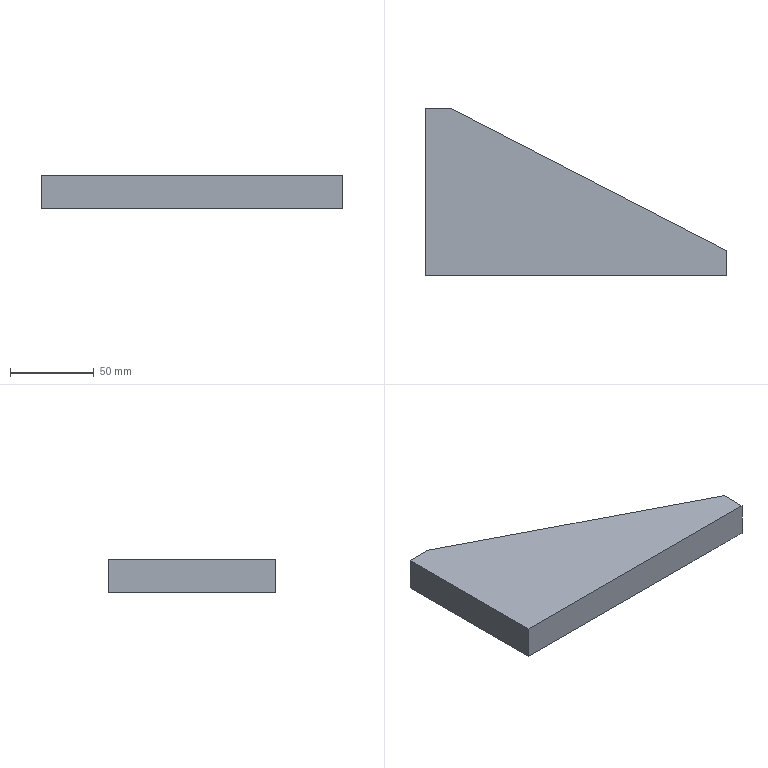Part | SolidWorks | features Extrusion 1 | 1 solid | 7 faces | box 180 x 100 x 20 mm | volume 219750 mm3 | plane 7
STEP:
#1=CARTESIAN_POINT('',(0.,0.,0.));
#2=VERTEX_POINT('',#1);
#3=CARTESIAN_POINT('',(180.,0.,0.));
#4=VERTEX_POINT('',#3);
#5=CARTESIAN_POINT('',(180.,0.,0.));
#6=DIRECTION('',(1.,0.,0.));
#7=VECTOR('',#6,1000.);
#8=LINE('',#5,#7);
#9=EDGE_CURVE('',#2,#4,#8,.T.);
#10=ORIENTED_EDGE('',*,*,#9,.T.);
#11=CARTESIAN_POINT('',(180.,0.,20.));
#12=VERTEX_POINT('',#11);
#13=CARTESIAN_POINT('',(180.,0.,20.));
#14=DIRECTION('',(0.,0.,-1.));
#15=VECTOR('',#14,1000.);
#16=LINE('',#13,#15);
#17=EDGE_CURVE('',#12,#4,#16,.T.);
#18=ORIENTED_EDGE('',*,*,#17,.F.);
#19=CARTESIAN_POINT('',(0.,0.,20.));
#20=VERTEX_POINT('',#19);
#21=CARTESIAN_POINT('',(180.,0.,20.));
#22=DIRECTION('',(1.,0.,0.));
#23=VECTOR('',#22,1000.);
#24=LINE('',#21,#23);
#25=EDGE_CURVE('',#20,#12,#24,.T.);
#26=ORIENTED_EDGE('',*,*,#25,.F.);
#27=CARTESIAN_POINT('',(0.,0.,20.));
#28=DIRECTION('',(0.,0.,-1.));
#29=VECTOR('',#28,1000.);
#30=LINE('',#27,#29);
#31=EDGE_CURVE('',#20,#2,#30,.T.);
#32=ORIENTED_EDGE('',*,*,#31,.T.);
#33=EDGE_LOOP('',(#10,#18,#26,#32));
#34=FACE_OUTER_BOUND('',#33,.T.);
#35=CARTESIAN_POINT('',(180.,0.,20.));
#36=DIRECTION('',(0.,1.,0.));
#37=DIRECTION('',(-1.,0.,0.));
#38=AXIS2_PLACEMENT_3D('',#35,#36,#37);
#39=PLANE('',#38);
#40=ADVANCED_FACE('',(#34),#39,.F.);
#41=CARTESIAN_POINT('',(180.,15.,0.));
#42=VERTEX_POINT('',#41);
#43=CARTESIAN_POINT('',(180.,15.,0.));
#44=DIRECTION('',(0.,1.,0.));
#45=VECTOR('',#44,1000.);
#46=LINE('',#43,#45);
#47=EDGE_CURVE('',#4,#42,#46,.T.);
#48=ORIENTED_EDGE('',*,*,#47,.T.);
#49=CARTESIAN_POINT('',(180.,15.,20.));
#50=VERTEX_POINT('',#49);
#51=CARTESIAN_POINT('',(180.,15.,20.));
#52=DIRECTION('',(0.,0.,-1.));
#53=VECTOR('',#52,1000.);
#54=LINE('',#51,#53);
#55=EDGE_CURVE('',#50,#42,#54,.T.);
#56=ORIENTED_EDGE('',*,*,#55,.F.);
#57=CARTESIAN_POINT('',(180.,15.,20.));
#58=DIRECTION('',(0.,1.,0.));
#59=VECTOR('',#58,1000.);
#60=LINE('',#57,#59);
#61=EDGE_CURVE('',#12,#50,#60,.T.);
#62=ORIENTED_EDGE('',*,*,#61,.F.);
#63=ORIENTED_EDGE('',*,*,#17,.T.);
#64=EDGE_LOOP('',(#48,#56,#62,#63));
#65=FACE_OUTER_BOUND('',#64,.T.);
#66=CARTESIAN_POINT('',(180.,15.,20.));
#67=DIRECTION('',(-1.,0.,0.));
#68=DIRECTION('',(0.,0.,1.));
#69=AXIS2_PLACEMENT_3D('',#66,#67,#68);
#70=PLANE('',#69);
#71=ADVANCED_FACE('',(#65),#70,.F.);
#72=CARTESIAN_POINT('',(15.,100.,0.));
#73=VERTEX_POINT('',#72);
#74=CARTESIAN_POINT('',(15.,100.,0.));
#75=DIRECTION('',(-0.889,0.458,0.));
#76=VECTOR('',#75,1000.);
#77=LINE('',#74,#76);
#78=EDGE_CURVE('',#42,#73,#77,.T.);
#79=ORIENTED_EDGE('',*,*,#78,.T.);
#80=CARTESIAN_POINT('',(15.,100.,20.));
#81=VERTEX_POINT('',#80);
#82=CARTESIAN_POINT('',(15.,100.,20.));
#83=DIRECTION('',(0.,0.,-1.));
#84=VECTOR('',#83,1000.);
#85=LINE('',#82,#84);
#86=EDGE_CURVE('',#81,#73,#85,.T.);
#87=ORIENTED_EDGE('',*,*,#86,.F.);
#88=CARTESIAN_POINT('',(15.,100.,20.));
#89=DIRECTION('',(-0.889,0.458,0.));
#90=VECTOR('',#89,1000.);
#91=LINE('',#88,#90);
#92=EDGE_CURVE('',#50,#81,#91,.T.);
#93=ORIENTED_EDGE('',*,*,#92,.F.);
#94=ORIENTED_EDGE('',*,*,#55,.T.);
#95=EDGE_LOOP('',(#79,#87,#93,#94));
#96=FACE_OUTER_BOUND('',#95,.T.);
#97=CARTESIAN_POINT('',(15.,100.,20.));
#98=DIRECTION('',(-0.458,-0.889,0.));
#99=DIRECTION('',(0.889,-0.458,0.));
#100=AXIS2_PLACEMENT_3D('',#97,#98,#99);
#101=PLANE('',#100);
#102=ADVANCED_FACE('',(#96),#101,.F.);
#103=CARTESIAN_POINT('',(0.,100.,0.));
#104=VERTEX_POINT('',#103);
#105=CARTESIAN_POINT('',(0.,100.,0.));
#106=DIRECTION('',(-1.,0.,0.));
#107=VECTOR('',#106,1000.);
#108=LINE('',#105,#107);
#109=EDGE_CURVE('',#73,#104,#108,.T.);
#110=ORIENTED_EDGE('',*,*,#109,.T.);
#111=CARTESIAN_POINT('',(0.,100.,20.));
#112=VERTEX_POINT('',#111);
#113=CARTESIAN_POINT('',(0.,100.,20.));
#114=DIRECTION('',(0.,0.,-1.));
#115=VECTOR('',#114,1000.);
#116=LINE('',#113,#115);
#117=EDGE_CURVE('',#112,#104,#116,.T.);
#118=ORIENTED_EDGE('',*,*,#117,.F.);
#119=CARTESIAN_POINT('',(0.,100.,20.));
#120=DIRECTION('',(-1.,0.,0.));
#121=VECTOR('',#120,1000.);
#122=LINE('',#119,#121);
#123=EDGE_CURVE('',#81,#112,#122,.T.);
#124=ORIENTED_EDGE('',*,*,#123,.F.);
#125=ORIENTED_EDGE('',*,*,#86,.T.);
#126=EDGE_LOOP('',(#110,#118,#124,#125));
#127=FACE_OUTER_BOUND('',#126,.T.);
#128=CARTESIAN_POINT('',(0.,100.,20.));
#129=DIRECTION('',(0.,-1.,0.));
#130=DIRECTION('',(0.,0.,-1.));
#131=AXIS2_PLACEMENT_3D('',#128,#129,#130);
#132=PLANE('',#131);
#133=ADVANCED_FACE('',(#127),#132,.F.);
#134=CARTESIAN_POINT('',(0.,0.,0.));
#135=DIRECTION('',(0.,-1.,0.));
#136=VECTOR('',#135,1000.);
#137=LINE('',#134,#136);
#138=EDGE_CURVE('',#104,#2,#137,.T.);
#139=ORIENTED_EDGE('',*,*,#138,.T.);
#140=ORIENTED_EDGE('',*,*,#31,.F.);
#141=CARTESIAN_POINT('',(0.,0.,20.));
#142=DIRECTION('',(0.,-1.,0.));
#143=VECTOR('',#142,1000.);
#144=LINE('',#141,#143);
#145=EDGE_CURVE('',#112,#20,#144,.T.);
#146=ORIENTED_EDGE('',*,*,#145,.F.);
#147=ORIENTED_EDGE('',*,*,#117,.T.);
#148=EDGE_LOOP('',(#139,#140,#146,#147));
#149=FACE_OUTER_BOUND('',#148,.T.);
#150=CARTESIAN_POINT('',(0.,0.,20.));
#151=DIRECTION('',(1.,0.,0.));
#152=DIRECTION('',(0.,0.,-1.));
#153=AXIS2_PLACEMENT_3D('',#150,#151,#152);
#154=PLANE('',#153);
#155=ADVANCED_FACE('',(#149),#154,.F.);
#156=ORIENTED_EDGE('',*,*,#25,.T.);
#157=ORIENTED_EDGE('',*,*,#61,.T.);
#158=ORIENTED_EDGE('',*,*,#92,.T.);
#159=ORIENTED_EDGE('',*,*,#123,.T.);
#160=ORIENTED_EDGE('',*,*,#145,.T.);
#161=EDGE_LOOP('',(#156,#157,#158,#159,#160));
#162=FACE_OUTER_BOUND('',#161,.T.);
#163=CARTESIAN_POINT('',(0.,0.,20.));
#164=DIRECTION('',(0.,0.,-1.));
#165=DIRECTION('',(-1.,0.,0.));
#166=AXIS2_PLACEMENT_3D('',#163,#164,#165);
#167=PLANE('',#166);
#168=ADVANCED_FACE('',(#162),#167,.F.);
#169=ORIENTED_EDGE('',*,*,#9,.F.);
#170=ORIENTED_EDGE('',*,*,#138,.F.);
#171=ORIENTED_EDGE('',*,*,#109,.F.);
#172=ORIENTED_EDGE('',*,*,#78,.F.);
#173=ORIENTED_EDGE('',*,*,#47,.F.);
#174=EDGE_LOOP('',(#169,#170,#171,#172,#173));
#175=FACE_OUTER_BOUND('',#174,.T.);
#176=CARTESIAN_POINT('',(0.,0.,0.));
#177=DIRECTION('',(0.,0.,-1.));
#178=DIRECTION('',(-1.,0.,0.));
#179=AXIS2_PLACEMENT_3D('',#176,#177,#178);
#180=PLANE('',#179);
#181=ADVANCED_FACE('',(#175),#180,.T.);
#182=CLOSED_SHELL('',(#40,#71,#102,#133,#155,#168,#181));
#183=MANIFOLD_SOLID_BREP('',#182);
#184=CARTESIAN_POINT('',(0.,0.,0.));
#185=DIRECTION('',(0.,0.,1.));
#186=DIRECTION('',(1.,0.,0.));
#187=AXIS2_PLACEMENT_3D('',#184,#185,#186);
#188=(LENGTH_UNIT()NAMED_UNIT(*)SI_UNIT(.MILLI.,.METRE.));
#189=UNCERTAINTY_MEASURE_WITH_UNIT(LENGTH_MEASURE(0.00001),#188,'','');
#190=(NAMED_UNIT(*)PLANE_ANGLE_UNIT()SI_UNIT($,.RADIAN.));
#191=(NAMED_UNIT(*)SI_UNIT($,.STERADIAN.)SOLID_ANGLE_UNIT());
#192=(GEOMETRIC_REPRESENTATION_CONTEXT(3)GLOBAL_UNCERTAINTY_ASSIGNED_CONTEXT((#189))GLOBAL_UNIT_ASSIGNED_CONTEXT((#188,#190,#191))REPRESENTATION_CONTEXT('',''));
#193=ADVANCED_BREP_SHAPE_REPRESENTATION('',(#183,#187),#192);